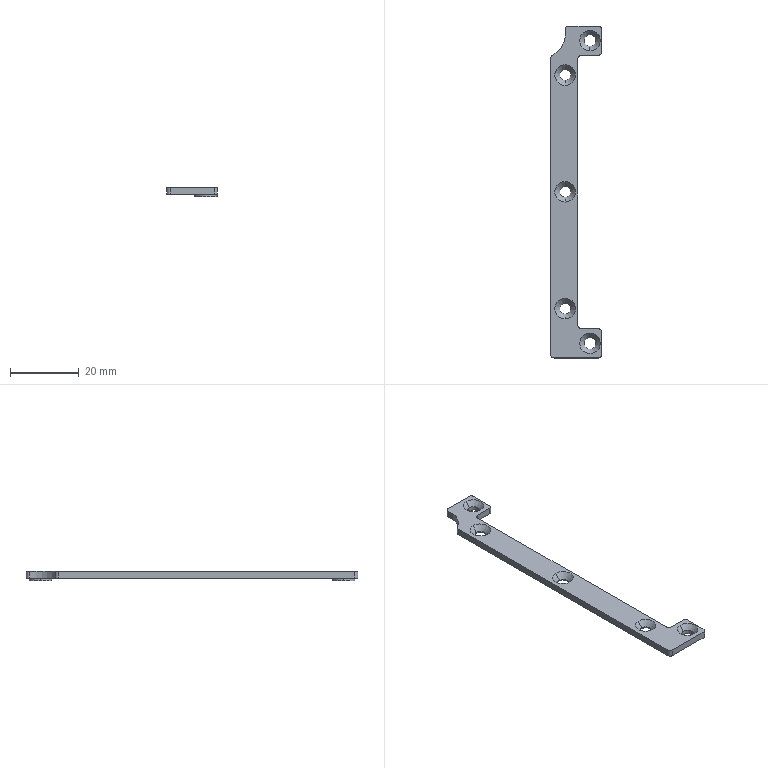NC program | NX | posted with a generic post | part box 14.723 x 96.5 x 2.7 mm
Whole program:
N10 G17 G21 G94 G90
(FLOOR_WALL , TOOL : D6)
N12 T06 M6
N14 G54
N16 G17 G0 G90 X-57.75 Y10.858 S9500 M3
N18 G43 Z30. H6
N20 Z3.
N22 G94 G1 Z0. F1500.
N24 X-54.75
N26 X54.75
N28 Y8.098
N30 X-54.75
N32 Y5.338
N34 X54.75
N36 Y2.578
N38 X-54.75
N40 Y-0.181
N42 X54.75
N44 Y-2.941
N46 X-54.75
N48 Y-4.253
N50 Y-5.701
N52 X54.75
N54 Y-8.461
N56 X-54.75
N58 X-57.75
N60 Z3.
N62 G0 Z30.
N64 M5
(DRILLING , TOOL : D6A45)
N66 T07 M6
N68 G54
N70 G17 G0 G90 X44. Y-4.061 S5000 M3
N72 G43 Z30. H7
N74 G94 G81 G98 Z-3. F250. R3.
N76 X34. Y3.15
N78 X0.05
N80 X-33.9
N82 X-44. Y-4.061
N84 G80
N86 G0 X-44. Y-4.061 Z30.
N88 M5
(CAVITY_MILL , TOOL : D4)
N90 T04 M6
N92 G54
N94 G17 G0 G90 X2.078 Y-13.659 S9500 M3
N96 G43 Z30. H4
N98 Z0.614
N100 G95 G1 Z-0.386 F1.579
N102 X0.866 Y-11.559
N104 G3 X0. Y-11.059 R1.
N106 G94 G1 X-51.746 F2500.
N108 G2 X-51.947 Y-10.865 R0.205
N110 G1 Y10.866
N112 G2 X-51.747 Y11.058 R0.204
N114 G1 X51.747
N116 G2 X51.948 Y10.865 R0.204
N118 G1 Y5.241
N120 X49.148
N122 G3 X46.771 Y5.74 R3.66
N124 G2 X42.006 Y8.138 R4.74
N126 G1 X41.936 Y8.258
N128 X49.148
N130 Y5.241
N132 X51.948
N134 Y-10.865
N136 G2 X51.746 Y-11.059 R0.205
N138 G1 X0.
N140 Y-8.259
N142 X-37.535
N144 G3 X-37.09 Y-6.561 R3.46
N146 G1 Y-3.221
N148 X37.09
N150 Y-6.561
N152 G3 X37.535 Y-8.259 R3.46
N154 G1 X38.023 Y-7.984
N156 G2 X37.65 Y-6.561 R2.9
N158 G1 Y-2.661
N160 X-37.65
N162 Y-6.561
N164 G2 X-40.55 Y-9.461 R2.9
N166 G1 X-47.45
N168 G2 X-50.35 Y-6.561 R2.9
N170 G1 Y6.361
N172 G2 X-47.25 Y9.461 R3.1
N174 G1 X38.806
N176 G2 X41.516 Y7.866 R3.1
N178 G3 X46.844 Y5.184 R5.3
N180 G2 X50.35 Y2.111 R3.1
N182 G1 Y-6.561
N184 G2 X47.45 Y-9.461 R2.9
N186 G1 X40.55
N188 G2 X38.023 Y-7.984 R2.9
N190 G1 X37.535 Y-8.259
N192 X0.
N194 Y-6.459
N196 X-35.29
N198 Y-5.021
N200 X35.29
N202 Y-6.459
N204 X0.
N206 G3 X-0.866 Y-6.959 R1.
N208 G1 Z0.614
N210 G0 Z30.
N212 X2.078 Y-13.659
N214 Z0.229
N216 G95 G1 Z-0.771 F1.579
N218 X0.866 Y-11.559
N220 G3 X0. Y-11.059 R1.
N222 G94 G1 X-51.746 F2500.
N224 G2 X-51.948 Y-10.865 R0.205
N226 G1 Y10.865
N228 G2 X-51.746 Y11.058 R0.204
N230 G1 X51.747
N232 G2 X51.948 Y10.865 R0.205
N234 G1 Y5.24
N236 X49.148
N238 G3 X46.771 Y5.74 R3.66
N240 G2 X42.006 Y8.138 R4.74
N242 G1 X41.936 Y8.258
N244 X49.148
N246 Y5.24
N248 X51.948
N250 Y-10.865
N252 G2 X51.746 Y-11.059 R0.206
N254 G1 X0.
N256 Y-8.259
N258 X-37.535
N260 G3 X-37.09 Y-6.561 R3.46
N262 G1 Y-3.221
N264 X37.09
N266 Y-6.561
N268 G3 X37.535 Y-8.259 R3.46
N270 G1 X38.023 Y-7.984
N272 G2 X37.65 Y-6.561 R2.9
N274 G1 Y-2.661
N276 X-37.65
N278 Y-6.561
N280 G2 X-40.55 Y-9.461 R2.9
N282 G1 X-47.45
N284 G2 X-50.35 Y-6.561 R2.9
N286 G1 Y6.361
N288 G2 X-47.25 Y9.461 R3.1
N290 G1 X38.806
N292 G2 X41.516 Y7.866 R3.1
N294 G3 X46.844 Y5.184 R5.3
N296 G2 X50.35 Y2.111 R3.1
N298 G1 Y-6.561
N300 G2 X47.45 Y-9.461 R2.9
N302 G1 X40.55
N304 G2 X38.023 Y-7.984 R2.9
N306 G1 X37.535 Y-8.259
N308 X0.
N310 Y-6.459
N312 X-35.29
N314 Y-5.021
N316 X35.29
N318 Y-6.459
N320 X0.
N322 G3 X-0.866 Y-6.959 R1.
N324 G1 Z0.229
N326 G0 X2.078 Y-13.66 Z-0.157
N328 G95 G1 Z-1.157 F1.579
N330 X0.866 Y-11.56
N332 G3 X0. Y-11.06 R1.
N334 G94 G1 X-51.746 F2500.
N336 G2 X-51.948 Y-10.865 R0.206
N338 G1 Y10.865
N340 G2 X-51.746 Y11.059 R0.205
N342 G1 X51.747
N344 G2 X51.949 Y10.865 R0.205
N346 G1 Y5.24
N348 X49.149
N350 G3 X46.771 Y5.74 R3.66
N352 G2 X42.006 Y8.138 R4.74
N354 G1 X41.936 Y8.259
N356 X49.149
N358 Y5.24
N360 X51.949
N362 Y-10.865
N364 G2 X51.746 Y-11.06 R0.206
N366 G1 X0.
N368 Y-8.26
N370 X-37.536
N372 G3 X-37.09 Y-6.561 R3.46
N374 G1 Y-3.221
N376 X37.09
N378 Y-6.561
N380 G3 X37.536 Y-8.26 R3.46
N382 G1 X38.023 Y-7.985
N384 G2 X37.65 Y-6.561 R2.9
N386 G1 Y-2.661
N388 X-37.65
N390 Y-6.561
N392 G2 X-40.55 Y-9.461 R2.9
N394 G1 X-47.45
N396 G2 X-50.35 Y-6.561 R2.9
N398 G1 Y6.361
N400 G2 X-47.25 Y9.461 R3.1
N402 G1 X38.806
N404 G2 X41.516 Y7.866 R3.1
N406 G3 X46.844 Y5.184 R5.3
N408 G2 X50.35 Y2.111 R3.1
N410 G1 Y-6.561
N412 G2 X47.45 Y-9.461 R2.9
N414 G1 X40.55
N416 G2 X38.023 Y-7.985 R2.9
N418 G1 X37.536 Y-8.26
N420 X0.
N422 Y-6.46
N424 X-35.29
N426 Y-5.021
N428 X35.29
N430 Y-6.46
N432 X0.
N434 G3 X-0.866 Y-6.96 R1.
N436 G1 Z-0.157
N438 G0 X2.078 Y-13.66 Z-0.543
N440 G95 G1 Z-1.543 F1.579
N442 X0.866 Y-11.56
N444 G3 X0. Y-11.06 R1.
N446 G94 G1 X-51.745 F2500.
N448 G2 X-51.948 Y-10.865 R0.206
N450 G1 Y10.865
N452 G2 X-51.746 Y11.059 R0.205
N454 G1 X51.746
N456 G2 X51.949 Y10.865 R0.206
N458 G1 Y5.24
N460 X49.149
N462 G3 X46.771 Y5.74 R3.66
N464 G2 X42.006 Y8.138 R4.74
N466 G1 X41.936 Y8.259
N468 X49.149
N470 Y5.24
N472 X51.949
N474 Y-10.865
N476 G2 X51.745 Y-11.06 R0.207
N478 G1 X0.
N480 Y-8.26
N482 X-37.536
N484 G3 X-37.09 Y-6.561 R3.46
N486 G1 Y-3.221
N488 X37.09
N490 Y-6.561
N492 G3 X37.536 Y-8.26 R3.46
N494 G1 X38.024 Y-7.985
N496 G2 X37.65 Y-6.561 R2.9
N498 G1 Y-2.661
N500 X-37.65
N502 Y-6.561
N504 G2 X-40.55 Y-9.461 R2.9
N506 G1 X-47.45
N508 G2 X-50.35 Y-6.561 R2.9
N510 G1 Y6.361
N512 G2 X-47.25 Y9.461 R3.1
N514 G1 X38.806
N516 G2 X41.516 Y7.866 R3.1
N518 G3 X46.844 Y5.184 R5.3
N520 G2 X50.35 Y2.111 R3.1
N522 G1 Y-6.561
N524 G2 X47.45 Y-9.461 R2.9
N526 G1 X40.55
N528 G2 X38.024 Y-7.985 R2.9
N530 G1 X37.536 Y-8.26
N532 X0.
N534 Y-6.46
N536 X-35.29
N538 Y-5.021
N540 X35.29
N542 Y-6.46
N544 X0.
N546 G3 X-0.866 Y-6.96 R1.
N548 G1 Z-0.543
N550 G0 X2.078 Y-13.66 Z-0.929
N552 G95 G1 Z-1.929 F1.579
N554 X0.866 Y-11.56
N556 G3 X0. Y-11.06 R1.
N558 G94 G1 X-51.745 F2500.
N560 G2 X-51.948 Y-10.865 R0.207
N562 G1 Y10.865
N564 G2 X-51.746 Y11.059 R0.205
N566 G1 X51.746
N568 G2 X51.949 Y10.865 R0.206
N570 G1 Y5.24
N572 X49.149
N574 G3 X46.771 Y5.74 R3.66
N576 G2 X42.006 Y8.138 R4.74
N578 G1 X41.936 Y8.259
N580 X49.149
N582 Y5.24
N584 X51.949
N586 Y-10.865
N588 G2 X51.745 Y-11.06 R0.208
N590 G1 X0.
N592 Y-8.26
N594 X-37.536
N596 G3 X-37.09 Y-6.561 R3.46
N598 G1 Y-3.221
N600 X37.09
N602 Y-6.561
N604 G3 X37.536 Y-8.26 R3.46
N606 G1 X38.024 Y-7.985
N608 G2 X37.65 Y-6.561 R2.9
N610 G1 Y-2.661
N612 X-37.65
N614 Y-6.561
N616 G2 X-40.55 Y-9.461 R2.9
N618 G1 X-47.45
N620 G2 X-50.35 Y-6.561 R2.9
N622 G1 Y6.361
N624 G2 X-47.25 Y9.461 R3.1
N626 G1 X38.806
N628 G2 X41.516 Y7.866 R3.1
N630 G3 X46.844 Y5.184 R5.3
N632 G2 X50.35 Y2.111 R3.1
N634 G1 Y-6.561
N636 G2 X47.45 Y-9.461 R2.9
N638 G1 X40.55
N640 G2 X38.024 Y-7.985 R2.9
N642 G1 X37.536 Y-8.26
N644 X0.
N646 Y-6.46
N648 X-35.29
N650 Y-5.021
N652 X35.29
N654 Y-6.46
N656 X0.
N658 G3 X-0.866 Y-6.96 R1.
N660 G1 Z-0.929
N662 G0 X2.078 Y-13.661 Z-1.314
N664 G95 G1 Z-2.314 F1.579
N666 X0.866 Y-11.561
N668 G3 X0. Y-11.061 R1.
N670 G94 G1 X-51.745 F2500.
N672 G2 X-51.948 Y-10.865 R0.207
N674 G1 Y10.865
N676 G2 X-51.746 Y11.059 R0.205
N678 G1 X51.746
N680 G2 X51.949 Y10.864 R0.206
N682 G1 Y5.24
N684 X49.149
N686 G3 X46.771 Y5.74 R3.66
N688 G2 X42.006 Y8.138 R4.74
N690 G1 X41.936 Y8.259
N692 X49.149
N694 Y5.24
N696 X51.949
N698 Y-10.864
N700 G2 X51.745 Y-11.061 R0.208
N702 G1 X0.
N704 Y-8.261
N706 X-37.536
N708 G3 X-37.09 Y-6.561 R3.46
N710 G1 Y-3.221
N712 X37.09
N714 Y-6.561
N716 G3 X37.536 Y-8.261 R3.46
N718 G1 X38.024 Y-7.986
N720 G2 X37.65 Y-6.561 R2.9
N722 G1 Y-2.661
N724 X-37.65
N726 Y-6.561
N728 G2 X-40.55 Y-9.461 R2.9
N730 G1 X-47.45
N732 G2 X-50.35 Y-6.561 R2.9
N734 G1 Y6.361
N736 G2 X-47.25 Y9.461 R3.1
N738 G1 X38.806
N740 G2 X41.516 Y7.866 R3.1
N742 G3 X46.844 Y5.184 R5.3
N744 G2 X50.35 Y2.111 R3.1
N746 G1 Y-6.561
N748 G2 X47.45 Y-9.461 R2.9
N750 G1 X40.55
N752 G2 X38.024 Y-7.986 R2.9
N754 G1 X37.536 Y-8.261
N756 X0.
N758 Y-6.461
N760 X-35.29
N762 Y-5.021
N764 X35.29
N766 Y-6.461
N768 X0.
N770 G3 X-0.866 Y-6.961 R1.
N772 G1 Z-1.314
N774 G0 X2.078 Y-13.661 Z-1.7
N776 G95 G1 Z-2.7 F1.579
N778 X0.866 Y-11.561
N780 G3 X0. Y-11.061 R1.
N782 G94 G1 X-51.745 F2500.
N784 G2 X-51.948 Y-10.865 R0.208
N786 G1 Y10.865
N788 G2 X-51.746 Y11.059 R0.206
N790 G1 X51.746
N792 G2 X51.95 Y10.864 R0.207
N794 G1 Y5.239
N796 X49.15
N798 G3 X46.771 Y5.74 R3.66
N800 G2 X42.006 Y8.138 R4.74
N802 G1 X41.935 Y8.259
N804 X49.15
N806 Y5.239
N808 X51.95
N810 Y-10.864
N812 G2 X51.745 Y-11.061 R0.209
N814 G1 X0.
N816 Y-8.261
N818 X-37.536
N820 G3 X-37.09 Y-6.561 R3.46
N822 G1 Y-3.221
N824 X37.09
N826 Y-6.561
N828 G3 X37.536 Y-8.261 R3.46
N830 G1 X38.024 Y-7.986
N832 G2 X37.65 Y-6.561 R2.9
N834 G1 Y-2.661
N836 X-37.65
N838 Y-6.561
N840 G2 X-40.55 Y-9.461 R2.9
N842 G1 X-47.45
N844 G2 X-50.35 Y-6.561 R2.9
N846 G1 Y6.361
N848 G2 X-47.25 Y9.461 R3.1
N850 G1 X38.806
N852 G2 X41.516 Y7.866 R3.1
N854 G3 X46.844 Y5.184 R5.3
N856 G2 X50.35 Y2.111 R3.1
N858 G1 Y-6.561
N860 G2 X47.45 Y-9.461 R2.9
N862 G1 X40.55
N864 G2 X38.024 Y-7.986 R2.9
N866 G1 X37.536 Y-8.261
N868 X0.
N870 Y-6.461
N872 X-35.29
N874 Y-5.021
N876 X35.29
N878 Y-6.461
N880 X0.
N882 G3 X-0.866 Y-6.961 R1.
N884 G1 Z-1.7
N886 G0 Z30.
(CAVITY_MILL_COPY , TOOL : D4)
N888 X-48.217 Y10.036
N890 Z-1.7
N892 G95 G1 Z-2.7 F1.579
N894 X-48.116 Y9.861
N896 G3 X-47.25 Y9.361 R1.
N898 G94 G1 X38.806 F1200.
N900 G2 X41.429 Y7.818 R3.
N902 G3 X46.857 Y5.085 R5.4
N904 G2 X50.25 Y2.111 R3.
N906 G1 Y-6.561
N908 G2 X47.45 Y-9.361 R2.8
N910 G1 X40.55
N912 G2 X37.75 Y-6.561 R2.8
N914 G1 Y-2.561
N916 X-37.75
N918 Y-6.561
N920 G2 X-40.55 Y-9.361 R2.8
N922 G1 X-47.45
N924 G2 X-50.25 Y-6.561 R2.8
N926 G1 Y6.361
N928 G2 X-47.25 Y9.361 R3.
N930 G3 X-46.384 Y9.861 R1.
N932 G1 X-46.211 Y10.161
N934 Z-1.7
N936 G0 Z30.
N938 M5
(CAVITY_MILL_COPY_1 , TOOL : D2)
N940 T02 M6
N942 G54
N944 G17 G0 G90 X38.35 Y-3.66 S9500 M3
N946 G43 Z30. H2
N948 Z0.807
N950 G95 G1 Z-0.193 F1.579
N952 G3 X38.75 Y-2.86 R1.
N954 G94 G1 Y-1.561 F1200.
N956 X37.451
N958 G3 X36.651 Y-1.961 R1.
N960 G1 Z0.807
N962 G0 Z30.
N964 X38.35 Y-3.66
N966 Z0.614
N968 G95 G1 Z-0.386 F1.579
N970 G3 X38.75 Y-2.86 R1.
N972 G94 G1 Y-1.561 F1200.
N974 X37.451
N976 G3 X36.651 Y-1.961 R1.
N978 G1 Z0.614
N980 G0 Z30.
N982 X38.35 Y-3.66
N984 Z0.421
N986 G95 G1 Z-0.579 F1.579
N988 G3 X38.75 Y-2.86 R1.
N990 G94 G1 Y-1.561 F1200.
N992 X37.451
N994 G3 X36.651 Y-1.961 R1.
N996 G1 Z0.421
N998 G0 Z30.
N1000 X38.35 Y-3.66
N1002 Z0.229
N1004 G95 G1 Z-0.771 F1.579
N1006 G3 X38.75 Y-2.86 R1.
N1008 G94 G1 Y-1.561 F1200.
N1010 X37.451
N1012 G3 X36.651 Y-1.961 R1.
N1014 G1 Z0.229
N1016 G0 Z30.
N1018 X38.35 Y-3.66
N1020 Z0.036
N1022 G95 G1 Z-0.964 F1.579
N1024 G3 X38.75 Y-2.86 R1.
N1026 G94 G1 Y-1.561 F1200.
N1028 X37.451
N1030 G3 X36.651 Y-1.961 R1.
N1032 G1 Z0.036
N1034 G0 X38.35 Y-3.66 Z-0.157
N1036 G95 G1 Z-1.157 F1.579
N1038 G3 X38.75 Y-2.86 R1.
N1040 G94 G1 Y-1.561 F1200.
N1042 X37.451
N1044 G3 X36.651 Y-1.961 R1.
N1046 G1 Z-0.157
N1048 G0 X38.35 Y-3.66 Z-0.35
N1050 G95 G1 Z-1.35 F1.579
N1052 G3 X38.75 Y-2.86 R1.
N1054 G94 G1 Y-1.561 F1200.
N1056 X37.451
N1058 G3 X36.651 Y-1.961 R1.
N1060 G1 Z-0.35
N1062 G0 X38.35 Y-3.66 Z-0.543
N1064 G95 G1 Z-1.543 F1.579
N1066 G3 X38.75 Y-2.86 R1.
N1068 G94 G1 Y-1.561 F1200.
N1070 X37.451
N1072 G3 X36.651 Y-1.961 R1.
N1074 G1 Z-0.543
N1076 G0 X38.35 Y-3.66 Z-0.736
N1078 G95 G1 Z-1.736 F1.579
N1080 G3 X38.75 Y-2.86 R1.
N1082 G94 G1 Y-1.561 F1200.
N1084 X37.451
N1086 G3 X36.651 Y-1.961 R1.
N1088 G1 Z-0.736
N1090 G0 X38.35 Y-3.66 Z-0.929
N1092 G95 G1 Z-1.929 F1.579
N1094 G3 X38.75 Y-2.86 R1.
N1096 G94 G1 Y-1.561 F1200.
N1098 X37.451
N1100 G3 X36.651 Y-1.961 R1.
N1102 G1 Z-0.929
N1104 G0 X38.35 Y-3.654 Z-1.121
N1106 G95 G1 Z-2.121 F1.579
N1108 G3 X38.75 Y-2.854 R1.
N1110 G94 G1 Y-1.561 F1200.
N1112 X37.449
N1114 G3 X36.649 Y-1.961 R1.
N1116 G1 Z-1.121
N1118 G0 X38.35 Y-3.654 Z-1.314
N1120 G95 G1 Z-2.314 F1.579
N1122 G3 X38.75 Y-2.854 R1.
N1124 G94 G1 Y-1.561 F1200.
N1126 X37.449
N1128 G3 X36.649 Y-1.961 R1.
N1130 G1 Z-1.314
N1132 G0 X38.35 Y-3.654 Z-1.507
N1134 G95 G1 Z-2.507 F1.579
N1136 G3 X38.75 Y-2.854 R1.
N1138 G94 G1 Y-1.561 F1200.
N1140 X37.449
N1142 G3 X36.649 Y-1.961 R1.
N1144 G1 Z-1.507
N1146 G0 X38.35 Y-3.654 Z-1.7
N1148 G95 G1 Z-2.7 F1.579
N1150 G3 X38.75 Y-2.854 R1.
N1152 G94 G1 Y-1.561 F1200.
N1154 X37.449
N1156 G3 X36.649 Y-1.961 R1.
N1158 G1 Z-1.7
N1160 G0 Z30.
N1162 X-36.651
N1164 Z0.807
N1166 G95 G1 Z-0.193 F1.579
N1168 G3 X-37.451 Y-1.561 R1.
N1170 G94 G1 X-38.698 F1200.
N1172 X-38.752 Y-1.559
N1174 X-38.75 Y-1.575
N1176 Y-2.86
N1178 G3 X-38.35 Y-3.66 R1.
N1180 G1 Z0.807
N1182 G0 Z30.
N1184 X-36.651 Y-1.961
N1186 Z0.614
N1188 G95 G1 Z-0.386 F1.579
N1190 G3 X-37.451 Y-1.561 R1.
N1192 G94 G1 X-38.698 F1200.
N1194 X-38.752 Y-1.559
N1196 X-38.75 Y-1.575
N1198 Y-2.86
N1200 G3 X-38.35 Y-3.66 R1.
N1202 G1 Z0.614
N1204 G0 Z30.
N1206 X-36.651 Y-1.961
N1208 Z0.421
N1210 G95 G1 Z-0.579 F1.579
N1212 G3 X-37.451 Y-1.561 R1.
N1214 G94 G1 X-38.698 F1200.
N1216 X-38.752 Y-1.56
N1218 X-38.75 Y-1.575
N1220 Y-2.86
N1222 G3 X-38.35 Y-3.66 R1.
N1224 G1 Z0.421
N1226 G0 Z30.
N1228 X-36.651 Y-1.961
N1230 Z0.229
N1232 G95 G1 Z-0.771 F1.579
N1234 G3 X-37.451 Y-1.561 R1.
N1236 G94 G1 X-38.698 F1200.
N1238 X-38.751 Y-1.56
N1240 X-38.75 Y-1.575
N1242 Y-2.86
N1244 G3 X-38.35 Y-3.66 R1.
N1246 G1 Z0.229
N1248 G0 Z30.
N1250 X-36.651 Y-1.961
N1252 Z0.036
N1254 G95 G1 Z-0.964 F1.579
N1256 G3 X-37.451 Y-1.561 R1.
N1258 G94 G1 X-38.698 F1200.
N1260 X-38.751 Y-1.56
N1262 X-38.75 Y-1.575
N1264 Y-2.86
N1266 G3 X-38.35 Y-3.66 R1.
N1268 G1 Z0.036
N1270 G0 X-36.651 Y-1.961 Z-0.157
N1272 G95 G1 Z-1.157 F1.579
N1274 G3 X-37.451 Y-1.561 R1.
N1276 G94 G1 X-38.698 F1200.
N1278 X-38.751 Y-1.56
N1280 X-38.75 Y-2.86
N1282 G3 X-38.35 Y-3.66 R1.
N1284 G1 Z-0.157
N1286 G0 X-36.651 Y-1.961 Z-0.35
N1288 G95 G1 Z-1.35 F1.579
N1290 G3 X-37.451 Y-1.561 R1.
N1292 G94 G1 X-38.698 F1200.
N1294 X-38.751
N1296 X-38.75 Y-2.86
N1298 G3 X-38.35 Y-3.66 R1.
N1300 G1 Z-0.35
N1302 G0 X-36.651 Y-1.961 Z-0.543
N1304 G95 G1 Z-1.543 F1.579
N1306 G3 X-37.451 Y-1.561 R1.
N1308 G94 G1 X-38.698 F1200.
N1310 X-38.75
N1312 Y-2.86
N1314 G3 X-38.35 Y-3.66 R1.
N1316 G1 Z-0.543
N1318 G0 X-36.651 Y-1.961 Z-0.736
N1320 G95 G1 Z-1.736 F1.579
N1322 G3 X-37.451 Y-1.561 R1.
N1324 G94 G1 X-38.698 F1200.
N1326 X-38.75
N1328 Y-2.86
N1330 G3 X-38.35 Y-3.66 R1.
N1332 G1 Z-0.736
N1334 G0 X-36.651 Y-1.961 Z-0.929
N1336 G95 G1 Z-1.929 F1.579
N1338 G3 X-37.451 Y-1.561 R1.
N1340 G94 G1 X-38.75 F1200.
N1342 Y-2.86
N1344 G3 X-38.35 Y-3.66 R1.
N1346 G1 Z-0.929
N1348 G0 X-36.651 Y-1.961 Z-1.121
N1350 G95 G1 Z-2.121 F1.579
N1352 G3 X-37.451 Y-1.561 R1.
N1354 G94 G1 X-38.75 F1200.
N1356 Y-2.859
N1358 G3 X-38.35 Y-3.659 R1.
N1360 G1 Z-1.121
N1362 G0 X-36.651 Y-1.961 Z-1.314
N1364 G95 G1 Z-2.314 F1.579
N1366 G3 X-37.451 Y-1.561 R1.
N1368 G94 G1 X-38.75 F1200.
N1370 Y-2.859
N1372 G3 X-38.35 Y-3.659 R1.
N1374 G1 Z-1.314
N1376 G0 X-36.651 Y-1.961 Z-1.507
N1378 G95 G1 Z-2.507 F1.579
N1380 G3 X-37.451 Y-1.561 R1.
N1382 G94 G1 X-38.75 F1200.
N1384 Y-2.859
N1386 G3 X-38.35 Y-3.659 R1.
N1388 G1 Z-1.507
N1390 G0 X-36.651 Y-1.961 Z-1.7
N1392 G95 G1 Z-2.7 F1.579
N1394 G3 X-37.451 Y-1.561 R1.
N1396 G94 G1 X-38.75 F1200.
N1398 Y-2.859
N1400 G3 X-38.35 Y-3.659 R1.
N1402 G1 Z-1.7
N1404 G0 Z30.
(HOLE_MILLING , TOOL : D2)
N1406 X-44. Y-4.061
N1408 Z0.5
N1410 G3 X-44.35 Y-4.411 R0.35 F1250.
N1412 X-44. Y-4.761 R0.35
N1414 X-44. Y-4.761 Z0.3 I0. J0.7
N1416 X-44. Y-4.761 Z0.1 I0. J0.7
N1418 X-44. Y-4.761 Z-0.1 I0. J0.7
N1420 X-44. Y-4.761 Z-0.3 I0. J0.7
N1422 X-44. Y-4.761 Z-0.5 I0. J0.7
N1424 X-44. Y-4.761 Z-0.7 I0. J0.7
N1426 X-44. Y-4.761 Z-0.9 I0. J0.7
N1428 X-44. Y-4.761 Z-1.1 I0. J0.7
N1430 X-44. Y-4.761 Z-1.3 I0. J0.7
N1432 X-44. Y-4.761 Z-1.5 I0. J0.7
N1434 X-44. Y-4.761 Z-1.7 I0. J0.7
N1436 X-44. Y-4.761 Z-1.9 I0. J0.7
N1438 X-44. Y-4.761 Z-2.1 I0. J0.7
N1440 X-44. Y-4.761 Z-2.3 I0. J0.7
N1442 X-44. Y-4.761 Z-2.5 I0. J0.7
N1444 X-44. Y-4.761 Z-2.7 I0. J0.7
N1446 X-43.3 Y-4.061 R0.7
N1448 X-44. Y-4.761 R-0.7
N1450 X-43.65 Y-4.411 R0.35
N1452 X-44. Y-4.061 R0.35
N1454 G0 Z30.
N1456 X-33.9 Y3.15
N1458 Z0.5
N1460 G3 X-34.2 Y2.85 R0.3
N1462 X-33.9 Y2.55 R0.3
N1464 X-33.9 Y2.55 Z0.3 I0. J0.6
N1466 X-33.9 Y2.55 Z0.1 I0. J0.6
N1468 X-33.9 Y2.55 Z-0.1 I0. J0.6
N1470 X-33.9 Y2.55 Z-0.3 I0. J0.6
N1472 X-33.9 Y2.55 Z-0.5 I0. J0.6
N1474 X-33.9 Y2.55 Z-0.7 I0. J0.6
N1476 X-33.9 Y2.55 Z-0.9 I0. J0.6
N1478 X-33.9 Y2.55 Z-1.1 I0. J0.6
N1480 X-33.9 Y2.55 Z-1.3 I0. J0.6
N1482 X-33.9 Y2.55 Z-1.5 I0. J0.6
N1484 X-33.9 Y2.55 Z-1.7 I0. J0.6
N1486 X-33.9 Y2.55 Z-1.9 I0. J0.6
N1488 X-33.9 Y3.75 Z-2. I0. J0.6
N1490 X-34.5 Y3.15 R0.6
N1492 X-33.9 Y3.75 R-0.6
N1494 X-34.2 Y3.45 R0.3
N1496 X-33.9 Y3.15 R0.3
N1498 G0 Z30.
N1500 X0.05
N1502 Z0.5
N1504 G3 X-0.25 Y2.85 R0.3
N1506 X0.05 Y2.55 R0.3
N1508 X0.05 Y2.55 Z0.3 I0. J0.6
N1510 X0.05 Y2.55 Z0.1 I0. J0.6
N1512 X0.05 Y2.55 Z-0.1 I0. J0.6
N1514 X0.05 Y2.55 Z-0.3 I0. J0.6
N1516 X0.05 Y2.55 Z-0.5 I0. J0.6
N1518 X0.05 Y2.55 Z-0.7 I0. J0.6
N1520 X0.05 Y2.55 Z-0.9 I0. J0.6
N1522 X0.05 Y2.55 Z-1.1 I0. J0.6
N1524 X0.05 Y2.55 Z-1.3 I0. J0.6
N1526 X0.05 Y2.55 Z-1.5 I0. J0.6
N1528 X0.05 Y2.55 Z-1.7 I0. J0.6
N1530 X0.05 Y2.55 Z-1.9 I0. J0.6
N1532 X0.05 Y3.75 Z-2. I0. J0.6
N1534 X-0.55 Y3.15 R0.6
N1536 X0.05 Y3.75 R-0.6
N1538 X-0.25 Y3.45 R0.3
N1540 X0.05 Y3.15 R0.3
N1542 G0 Z30.
N1544 X34.
N1546 Z0.5
N1548 G3 X33.7 Y2.85 R0.3
N1550 X34. Y2.55 R0.3
N1552 X34. Y2.55 Z0.3 I0. J0.6
N1554 X34. Y2.55 Z0.1 I0. J0.6
N1556 X34. Y2.55 Z-0.1 I0. J0.6
N1558 X34. Y2.55 Z-0.3 I0. J0.6
N1560 X34. Y2.55 Z-0.5 I0. J0.6
N1562 X34. Y2.55 Z-0.7 I0. J0.6
N1564 X34. Y2.55 Z-0.9 I0. J0.6
N1566 X34. Y2.55 Z-1.1 I0. J0.6
N1568 X34. Y2.55 Z-1.3 I0. J0.6
N1570 X34. Y2.55 Z-1.5 I0. J0.6
N1572 X34. Y2.55 Z-1.7 I0. J0.6
N1574 X34. Y2.55 Z-1.9 I0. J0.6
N1576 X34. Y3.75 Z-2. I0. J0.6
N1578 X33.4 Y3.15 R0.6
N1580 X34. Y3.75 R-0.6
N1582 X33.7 Y3.45 R0.3
N1584 X34. Y3.15 R0.3
N1586 G0 Z30.
N1588 X44. Y-4.061
N1590 Z0.5
N1592 G3 X43.65 Y-4.411 R0.35
N1594 X44. Y-4.761 R0.35
N1596 X44. Y-4.761 Z0.3 I0. J0.7
N1598 X44. Y-4.761 Z0.1 I0. J0.7
N1600 X44. Y-4.761 Z-0.1 I0. J0.7
N1602 X44. Y-4.761 Z-0.3 I0. J0.7
N1604 X44. Y-4.761 Z-0.5 I0. J0.7
N1606 X44. Y-4.761 Z-0.7 I0. J0.7
N1608 X44. Y-4.761 Z-0.9 I0. J0.7
N1610 X44. Y-4.761 Z-1.1 I0. J0.7
N1612 X44. Y-4.761 Z-1.3 I0. J0.7
N1614 X44. Y-4.761 Z-1.5 I0. J0.7
N1616 X44. Y-4.761 Z-1.7 I0. J0.7
N1618 X44. Y-4.761 Z-1.9 I0. J0.7
N1620 X44. Y-4.761 Z-2.1 I0. J0.7
N1622 X44. Y-4.761 Z-2.3 I0. J0.7
N1624 X44. Y-4.761 Z-2.5 I0. J0.7
N1626 X44. Y-4.761 Z-2.7 I0. J0.7
N1628 X44.7 Y-4.061 R0.7
N1630 X44. Y-4.761 R-0.7
N1632 X44.35 Y-4.411 R0.35
N1634 X44. Y-4.061 R0.35
N1636 G0 Z30.
N1638 M5
(PLANAR_MILL , TOOL : D6A45)
N1640 T07 M6
N1642 G54
N1644 G17 G0 G90 X45.457 Y5.184 S9500 M3
N1646 G43 Z30. H7
N1648 Z0.5
N1650 G94 G1 Z-1. F1250.
N1652 X46.077 Y4.377
N1654 G3 X47.001 Y3.995 R1.
N1656 G2 X49.15 Y2.111 R1.9
N1658 G1 Y-6.561
N1660 G2 X47.45 Y-8.261 R1.7
N1662 G1 X40.55
N1664 G2 X38.85 Y-6.561 R1.7
N1666 G1 Y-1.561
N1668 X38.863 Y-1.496
N1670 X38.815 Y-1.449
N1672 X38.75 Y-1.461
N1674 X-38.75
N1676 X-38.815 Y-1.449
N1678 X-38.863 Y-1.496
N1680 X-38.85 Y-1.561
N1682 Y-6.561
N1684 G2 X-40.55 Y-8.261 R1.7
N1686 G1 X-47.45
N1688 G2 X-49.15 Y-6.561 R1.7
N1690 G1 Y6.361
N1692 G2 X-47.25 Y8.261 R1.9
N1694 G1 X38.806
N1696 G2 X40.467 Y7.284 R1.9
N1698 G3 X47.001 Y3.995 R6.5
N1700 X47.794 Y4.604 R1.
N1702 G1 X48.007 Y5.117
N1704 Z0.5
N1706 G0 Z30.
N1708 M5
N1710 M2